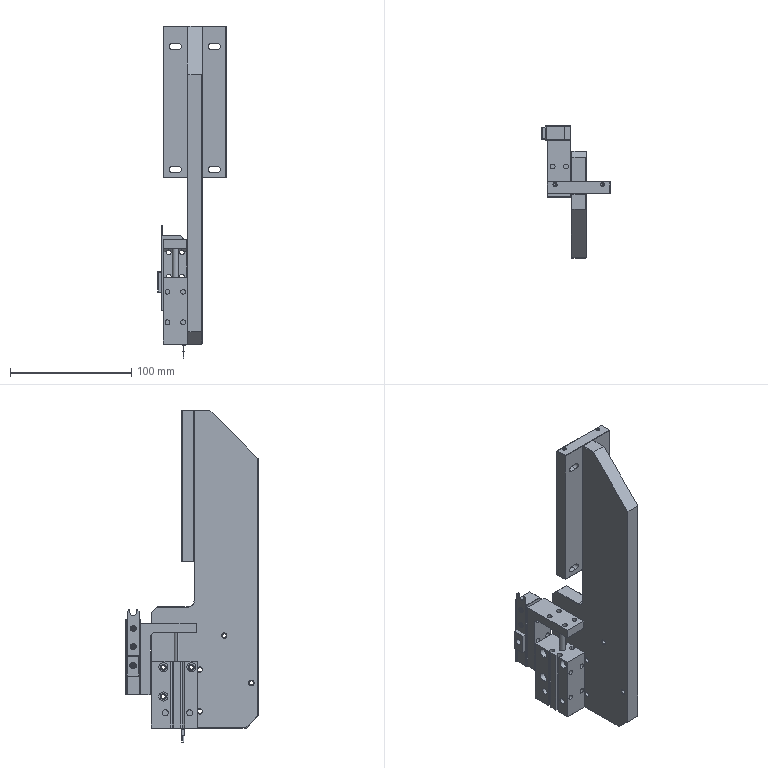Part | NX | 9 solids | 533 faces | box 56.5 x 109 x 273.5 mm | volume 321345 mm3 | cylinder 233 | plane 214 | cone 86 | commonest cylinder face diameters 2.5 x52 4 x48 5 x40 3.3 x22 4.5 x14 7.5 x12